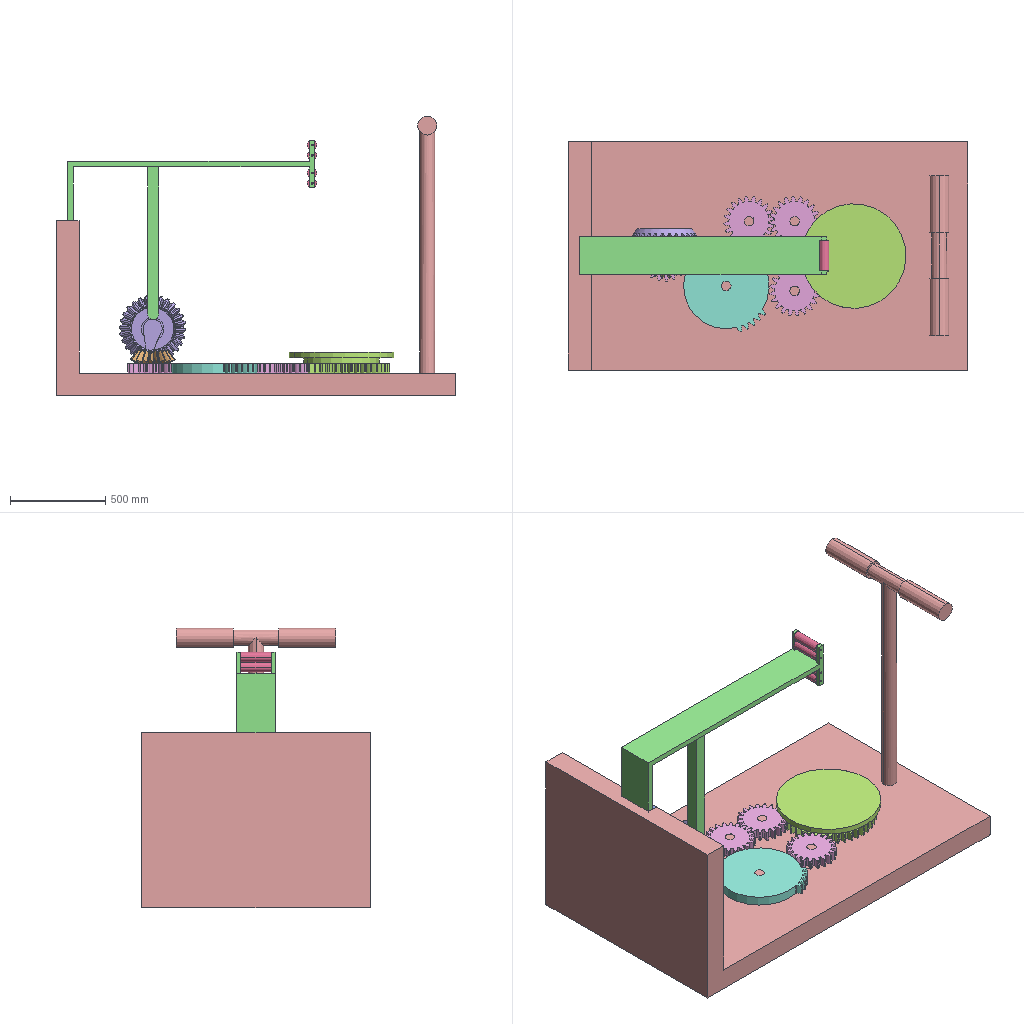Assembly | SolidWorks | 8 different items | 14 placed | box 2100 x 1200 x 1470 mm
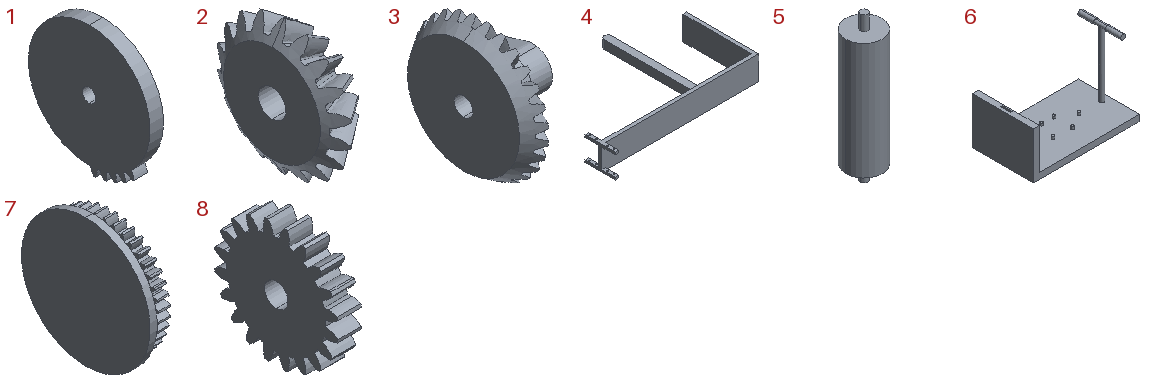Parts list (item | quantity | size | volume | features):
1 | x1 | 50 x 449.998 x 476.498 mm | 7974553 mm3 | features ICE 2, BaseBody 1
2 | x1 | 69.675 x 233.385 x 236.188 mm | 1498219 mm3 | features 3DProfileFeature 12, BlendCut 1, CirPattern 1, ICE 1, RefAxis 1, Revolution 1
3 | x1 | 180.071 x 347.819 x 347.819 mm | 5839211 mm3 | features 3DProfileFeature 12, ICE 2, BlendCut 1, CirPattern 1, RefAxis 1, Revolution 1
4 | x1 | 1300 x 940 x 200 mm | 14804394 mm3 | features ICE 3, Extrusion 1
5 | x4 | 50 x 50 x 200 mm | 317301 mm3 | features Extrusion 1, ICE 1, MirrorPattern 1
6 | x1 | 2100 x 1200 x 1470 mm | 421779830 mm3 | features ICE 12, Extrusion 1, MirrorPattern 1
7 | x1 | 110 x 550 x 550 mm | 19716444 mm3 | features BaseBody 1
8 | x4 | 50 x 261.706 x 261.706 mm | 2092246 mm3 | features BaseBody 1, ICE 1
Mates (type | each side: item.copy, entity, surface, feature):
Coincident | 6.1 face plane Boss-Extrude1 | 7.1 face plane Input1
Concentric | 6.1 face cylinder Boss-Extrude6 | 7.1 face cylinder Input1
Coincident | 6.1 face plane Boss-Extrude1 | 8.1 face plane Input1
Coincident | 6.1 face plane Boss-Extrude1 | 8.2 face plane Input1
Coincident | 6.1 select_type:24 | 8.1 face cylinder Input1
Coincident | 6.1 select_type:24 | 8.2 face cylinder Input1
Concentric | 6.1 face cylinder Boss-Extrude8 | 8.3 face cylinder Input1
Coincident | 6.1 face plane Boss-Extrude1 | 8.3 face plane Input1
Coincident | 6.1 face plane Boss-Extrude1 | 1.1 face plane Input1
Concentric | 6.1 face cylinder Boss-Extrude9 | 1.1 face cylinder Input1
GearDim | 8.1 select_type:24 | 7.1 select_type:24
GearDim | 8.1 select_type:24 | 8.3 select_type:24
GearDim | 7.1 select_type:24 | 8.2 select_type:24
GearDim | 8.3 select_type:24 | 1.1 select_type:24
Coincident | 6.1 face plane Boss-Extrude1 | 8.4 face plane Input1
Concentric | 6.1 face cylinder Boss-Extrude10 | 8.4 face cylinder Input1
GearDim | 8.4 select_type:24 | 1.1 select_type:24
Coincident | 8.4 face plane Input1 | 2.1 face plane Revolve1
Concentric | 8.4 face cylinder Input1 | 2.1 face cylinder Revolve1
Coincident | 2.1 select_type:25 | 3.1 select_type:25
Perpendicular | 2.1 face plane Revolve1 | 3.1 face plane Revolve1
Perpendicular | 6.1 face plane Boss-Extrude2 | 3.1 face plane Revolve1
GearDim | 2.1 select_type:24 | 3.1 select_type:24
Width | 4.1 face plane Boss-Extrude1 | 4.1 face plane Boss-Extrude1 | 6.1 face plane Cut-Extrude1 | 6.1 face plane Cut-Extrude1
Concentric | 4.1 face cylinder Cut-Extrude1 | 5.1 face cylinder Mirror1
Coincident | 4.1 face plane Boss-Extrude2 | 5.1 face plane Boss-Extrude1
Concentric | 4.1 face cylinder Cut-Extrude1 | 5.2 face cylinder Boss-Extrude2
Coincident | 4.1 face plane Boss-Extrude2 | 5.2 face plane Boss-Extrude1
CamTangent | 3.1 face surface:4009 Boss-Extrude2 | 4.1 face cylinder Boss-Extrude5
Coincident | 6.1 face plane Cut-Extrude1 | 4.1 face plane Boss-Extrude1
Coincident | 8.4 face plane Cut-Extrude1 | 2.1 face plane Cut-Extrude1